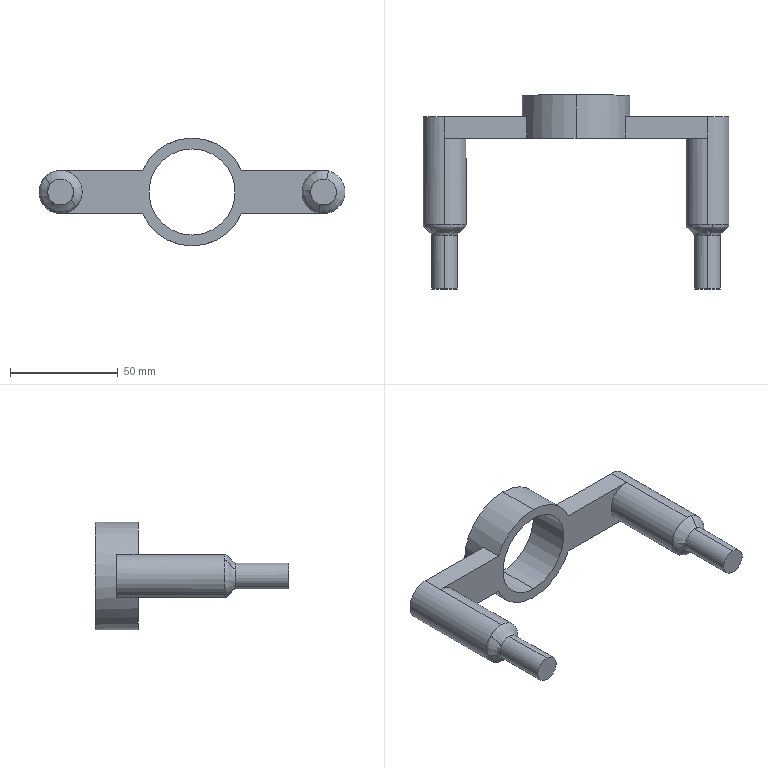Part | SolidWorks | features ICE 3, Blend 2, ExtruThin 1 | 1 solid | 26 faces | box 142.002 x 90 x 50 mm | volume 64913 mm3 | cylinder 12 | plane 10 | spline 4 | commonest cylinder face diameters 12 x4 20 x4 40 x2 50 x2